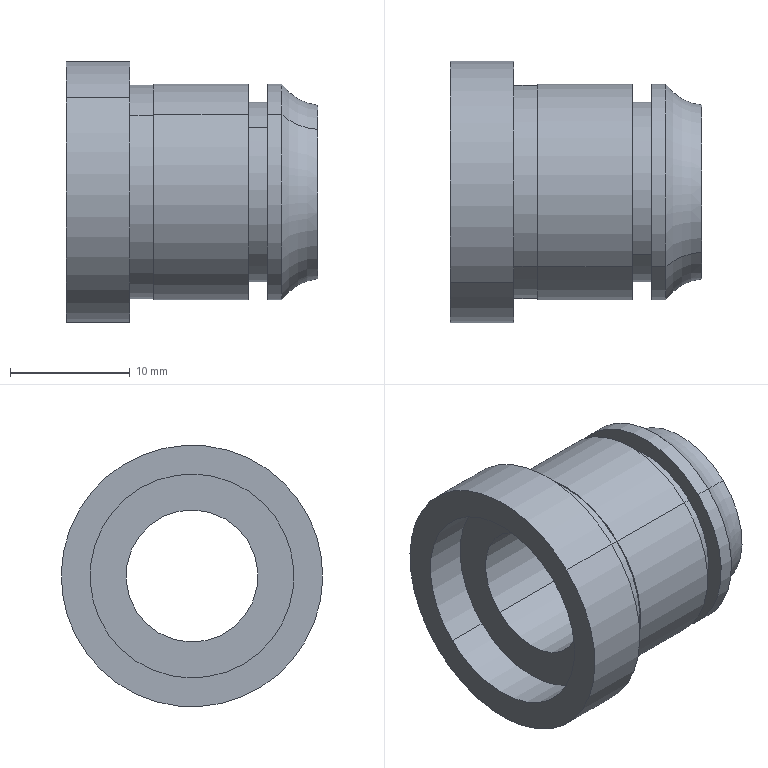Part | SolidWorks | features BaseBody 1 | 1 solid | 23 faces | box 21 x 21.8 x 21.8 mm | volume 3195 mm3 | cylinder 14 | plane 7 | torus 2 | commonest cylinder face diameters 18 x4 11 x2 15 x2 17 x2 17.8 x2 21.8 x2
STEP:
#1=CARTESIAN_POINT('',(-67.763,-3.139,-191.334));
#2=VERTEX_POINT('',#1);
#3=CARTESIAN_POINT('',(-67.763,6.932,-201.766));
#4=VERTEX_POINT('',#3);
#5=CARTESIAN_POINT('',(-67.763,1.896,-196.55));
#6=DIRECTION('',(1.,0.,0.));
#7=DIRECTION('',(0.,0.6945,-0.7195));
#8=AXIS2_PLACEMENT_3D('',#5,#6,#7);
#9=CIRCLE('',#8,7.25);
#10=EDGE_CURVE('',#2,#4,#9,.T.);
#11=ORIENTED_EDGE('',*,*,#10,.F.);
#12=CARTESIAN_POINT('',(-70.763,-4.355,-190.075));
#13=VERTEX_POINT('',#12);
#14=CARTESIAN_POINT('',(-67.447,-5.909,-188.465));
#15=DIRECTION('',(0.,0.7195,0.6945));
#16=DIRECTION('',(0.,-0.6945,0.7195));
#17=AXIS2_PLACEMENT_3D('',#14,#15,#16);
#18=CIRCLE('',#17,4.);
#19=EDGE_CURVE('',#2,#13,#18,.T.);
#20=ORIENTED_EDGE('',*,*,#19,.T.);
#21=CARTESIAN_POINT('',(-70.763,8.147,-203.025));
#22=VERTEX_POINT('',#21);
#23=CARTESIAN_POINT('',(-70.763,1.896,-196.55));
#24=DIRECTION('',(1.,0.,0.));
#25=DIRECTION('',(0.,0.6945,-0.7195));
#26=AXIS2_PLACEMENT_3D('',#23,#24,#25);
#27=CIRCLE('',#26,9.);
#28=EDGE_CURVE('',#13,#22,#27,.T.);
#29=ORIENTED_EDGE('',*,*,#28,.T.);
#30=CARTESIAN_POINT('',(-67.447,9.701,-204.635));
#31=DIRECTION('',(0.,-0.7195,-0.6945));
#32=DIRECTION('',(0.,0.6945,-0.7195));
#33=AXIS2_PLACEMENT_3D('',#30,#31,#32);
#34=CIRCLE('',#33,4.);
#35=EDGE_CURVE('',#4,#22,#34,.T.);
#36=ORIENTED_EDGE('',*,*,#35,.F.);
#37=EDGE_LOOP('',(#11,#20,#29,#36));
#38=FACE_OUTER_BOUND('',#37,.T.);
#39=CARTESIAN_POINT('',(-67.447,1.896,-196.55));
#40=DIRECTION('',(1.,0.,0.));
#41=DIRECTION('',(0.,0.6945,-0.7195));
#42=AXIS2_PLACEMENT_3D('',#39,#40,#41);
#43=TOROIDAL_SURFACE('',#42,11.238,4.);
#44=ADVANCED_FACE('',(#38),#43,.F.);
#45=CARTESIAN_POINT('',(-85.263,-1.924,-192.593));
#46=VERTEX_POINT('',#45);
#47=CARTESIAN_POINT('',(-85.263,5.716,-200.507));
#48=VERTEX_POINT('',#47);
#49=CARTESIAN_POINT('',(-85.263,1.896,-196.55));
#50=DIRECTION('',(1.,0.,0.));
#51=DIRECTION('',(0.,0.6945,-0.7195));
#52=AXIS2_PLACEMENT_3D('',#49,#50,#51);
#53=CIRCLE('',#52,5.5);
#54=EDGE_CURVE('',#46,#48,#53,.T.);
#55=ORIENTED_EDGE('',*,*,#54,.F.);
#56=CARTESIAN_POINT('',(-67.763,-1.924,-192.593));
#57=VERTEX_POINT('',#56);
#58=CARTESIAN_POINT('',(-87.763,-1.924,-192.593));
#59=DIRECTION('',(1.,0.,0.));
#60=VECTOR('',#59,1000.);
#61=LINE('',#58,#60);
#62=EDGE_CURVE('',#46,#57,#61,.T.);
#63=ORIENTED_EDGE('',*,*,#62,.T.);
#64=CARTESIAN_POINT('',(-67.763,5.716,-200.507));
#65=VERTEX_POINT('',#64);
#66=CARTESIAN_POINT('',(-67.763,1.896,-196.55));
#67=DIRECTION('',(1.,0.,0.));
#68=DIRECTION('',(0.,0.6945,-0.7195));
#69=AXIS2_PLACEMENT_3D('',#66,#67,#68);
#70=CIRCLE('',#69,5.5);
#71=EDGE_CURVE('',#57,#65,#70,.T.);
#72=ORIENTED_EDGE('',*,*,#71,.T.);
#73=CARTESIAN_POINT('',(-87.763,5.716,-200.507));
#74=DIRECTION('',(1.,0.,0.));
#75=VECTOR('',#74,1000.);
#76=LINE('',#73,#75);
#77=EDGE_CURVE('',#48,#65,#76,.T.);
#78=ORIENTED_EDGE('',*,*,#77,.F.);
#79=EDGE_LOOP('',(#55,#63,#72,#78));
#80=FACE_OUTER_BOUND('',#79,.T.);
#81=CARTESIAN_POINT('',(-87.763,1.896,-196.55));
#82=DIRECTION('',(1.,0.,0.));
#83=DIRECTION('',(0.,0.6945,-0.7195));
#84=AXIS2_PLACEMENT_3D('',#81,#82,#83);
#85=CYLINDRICAL_SURFACE('',#84,5.5);
#86=ADVANCED_FACE('',(#80),#85,.F.);
#87=CARTESIAN_POINT('',(-88.763,-4.007,-190.435));
#88=VERTEX_POINT('',#87);
#89=CARTESIAN_POINT('',(-88.763,7.8,-202.665));
#90=VERTEX_POINT('',#89);
#91=CARTESIAN_POINT('',(-88.763,1.896,-196.55));
#92=DIRECTION('',(1.,0.,0.));
#93=DIRECTION('',(0.,0.6945,-0.7195));
#94=AXIS2_PLACEMENT_3D('',#91,#92,#93);
#95=CIRCLE('',#94,8.5);
#96=EDGE_CURVE('',#88,#90,#95,.T.);
#97=ORIENTED_EDGE('',*,*,#96,.F.);
#98=CARTESIAN_POINT('',(-85.263,-4.007,-190.435));
#99=VERTEX_POINT('',#98);
#100=CARTESIAN_POINT('',(-87.763,-4.007,-190.435));
#101=DIRECTION('',(1.,0.,0.));
#102=VECTOR('',#101,1000.);
#103=LINE('',#100,#102);
#104=EDGE_CURVE('',#88,#99,#103,.T.);
#105=ORIENTED_EDGE('',*,*,#104,.T.);
#106=CARTESIAN_POINT('',(-85.263,7.8,-202.665));
#107=VERTEX_POINT('',#106);
#108=CARTESIAN_POINT('',(-85.263,1.896,-196.55));
#109=DIRECTION('',(1.,0.,0.));
#110=DIRECTION('',(0.,0.6945,-0.7195));
#111=AXIS2_PLACEMENT_3D('',#108,#109,#110);
#112=CIRCLE('',#111,8.5);
#113=EDGE_CURVE('',#99,#107,#112,.T.);
#114=ORIENTED_EDGE('',*,*,#113,.T.);
#115=CARTESIAN_POINT('',(-87.763,7.8,-202.665));
#116=DIRECTION('',(1.,0.,0.));
#117=VECTOR('',#116,1000.);
#118=LINE('',#115,#117);
#119=EDGE_CURVE('',#90,#107,#118,.T.);
#120=ORIENTED_EDGE('',*,*,#119,.F.);
#121=EDGE_LOOP('',(#97,#105,#114,#120));
#122=FACE_OUTER_BOUND('',#121,.T.);
#123=CARTESIAN_POINT('',(-87.763,1.896,-196.55));
#124=DIRECTION('',(1.,0.,0.));
#125=DIRECTION('',(0.,0.6945,-0.7195));
#126=AXIS2_PLACEMENT_3D('',#123,#124,#125);
#127=CYLINDRICAL_SURFACE('',#126,8.5);
#128=ADVANCED_FACE('',(#122),#127,.F.);
#129=CARTESIAN_POINT('',(-88.763,9.467,-204.392));
#130=VERTEX_POINT('',#129);
#131=CARTESIAN_POINT('',(-88.763,-5.674,-188.708));
#132=VERTEX_POINT('',#131);
#133=CARTESIAN_POINT('',(-88.763,1.896,-196.55));
#134=DIRECTION('',(1.,0.,0.));
#135=DIRECTION('',(0.,0.6945,-0.7195));
#136=AXIS2_PLACEMENT_3D('',#133,#134,#135);
#137=CIRCLE('',#136,10.9);
#138=EDGE_CURVE('',#130,#132,#137,.T.);
#139=ORIENTED_EDGE('',*,*,#138,.T.);
#140=CARTESIAN_POINT('',(-83.463,-5.674,-188.708));
#141=VERTEX_POINT('',#140);
#142=CARTESIAN_POINT('',(-87.763,-5.674,-188.708));
#143=DIRECTION('',(1.,0.,0.));
#144=VECTOR('',#143,1000.);
#145=LINE('',#142,#144);
#146=EDGE_CURVE('',#132,#141,#145,.T.);
#147=ORIENTED_EDGE('',*,*,#146,.T.);
#148=CARTESIAN_POINT('',(-83.463,9.467,-204.392));
#149=VERTEX_POINT('',#148);
#150=CARTESIAN_POINT('',(-83.463,1.896,-196.55));
#151=DIRECTION('',(1.,0.,0.));
#152=DIRECTION('',(0.,0.6945,-0.7195));
#153=AXIS2_PLACEMENT_3D('',#150,#151,#152);
#154=CIRCLE('',#153,10.9);
#155=EDGE_CURVE('',#149,#141,#154,.T.);
#156=ORIENTED_EDGE('',*,*,#155,.F.);
#157=CARTESIAN_POINT('',(-87.763,9.467,-204.392));
#158=DIRECTION('',(1.,0.,0.));
#159=VECTOR('',#158,1000.);
#160=LINE('',#157,#159);
#161=EDGE_CURVE('',#130,#149,#160,.T.);
#162=ORIENTED_EDGE('',*,*,#161,.F.);
#163=EDGE_LOOP('',(#139,#147,#156,#162));
#164=FACE_OUTER_BOUND('',#163,.T.);
#165=CARTESIAN_POINT('',(-87.763,1.896,-196.55));
#166=DIRECTION('',(1.,0.,0.));
#167=DIRECTION('',(0.,0.6945,-0.7195));
#168=AXIS2_PLACEMENT_3D('',#165,#166,#167);
#169=CYLINDRICAL_SURFACE('',#168,10.9);
#170=ADVANCED_FACE('',(#164),#169,.T.);
#171=CARTESIAN_POINT('',(-83.463,8.078,-202.953));
#172=VERTEX_POINT('',#171);
#173=CARTESIAN_POINT('',(-83.463,-4.285,-190.147));
#174=VERTEX_POINT('',#173);
#175=CARTESIAN_POINT('',(-83.463,1.896,-196.55));
#176=DIRECTION('',(1.,0.,0.));
#177=DIRECTION('',(0.,0.6945,-0.7195));
#178=AXIS2_PLACEMENT_3D('',#175,#176,#177);
#179=CIRCLE('',#178,8.9);
#180=EDGE_CURVE('',#172,#174,#179,.T.);
#181=ORIENTED_EDGE('',*,*,#180,.T.);
#182=CARTESIAN_POINT('',(-81.463,-4.285,-190.147));
#183=VERTEX_POINT('',#182);
#184=CARTESIAN_POINT('',(-87.763,-4.285,-190.147));
#185=DIRECTION('',(1.,0.,0.));
#186=VECTOR('',#185,1000.);
#187=LINE('',#184,#186);
#188=EDGE_CURVE('',#174,#183,#187,.T.);
#189=ORIENTED_EDGE('',*,*,#188,.T.);
#190=CARTESIAN_POINT('',(-81.463,8.078,-202.953));
#191=VERTEX_POINT('',#190);
#192=CARTESIAN_POINT('',(-81.463,1.896,-196.55));
#193=DIRECTION('',(1.,0.,0.));
#194=DIRECTION('',(0.,0.6945,-0.7195));
#195=AXIS2_PLACEMENT_3D('',#192,#193,#194);
#196=CIRCLE('',#195,8.9);
#197=EDGE_CURVE('',#191,#183,#196,.T.);
#198=ORIENTED_EDGE('',*,*,#197,.F.);
#199=CARTESIAN_POINT('',(-87.763,8.078,-202.953));
#200=DIRECTION('',(1.,0.,0.));
#201=VECTOR('',#200,1000.);
#202=LINE('',#199,#201);
#203=EDGE_CURVE('',#172,#191,#202,.T.);
#204=ORIENTED_EDGE('',*,*,#203,.F.);
#205=EDGE_LOOP('',(#181,#189,#198,#204));
#206=FACE_OUTER_BOUND('',#205,.T.);
#207=CARTESIAN_POINT('',(-87.763,1.896,-196.55));
#208=DIRECTION('',(1.,0.,0.));
#209=DIRECTION('',(0.,0.6945,-0.7195));
#210=AXIS2_PLACEMENT_3D('',#207,#208,#209);
#211=CYLINDRICAL_SURFACE('',#210,8.9);
#212=ADVANCED_FACE('',(#206),#211,.T.);
#213=CARTESIAN_POINT('',(-81.463,8.147,-203.025));
#214=VERTEX_POINT('',#213);
#215=CARTESIAN_POINT('',(-81.463,-4.355,-190.075));
#216=VERTEX_POINT('',#215);
#217=CARTESIAN_POINT('',(-81.463,1.896,-196.55));
#218=DIRECTION('',(1.,0.,0.));
#219=DIRECTION('',(0.,0.6945,-0.7195));
#220=AXIS2_PLACEMENT_3D('',#217,#218,#219);
#221=CIRCLE('',#220,9.);
#222=EDGE_CURVE('',#214,#216,#221,.T.);
#223=ORIENTED_EDGE('',*,*,#222,.T.);
#224=CARTESIAN_POINT('',(-73.563,-4.355,-190.075));
#225=VERTEX_POINT('',#224);
#226=CARTESIAN_POINT('',(-87.763,-4.355,-190.075));
#227=DIRECTION('',(1.,0.,0.));
#228=VECTOR('',#227,1000.);
#229=LINE('',#226,#228);
#230=EDGE_CURVE('',#216,#225,#229,.T.);
#231=ORIENTED_EDGE('',*,*,#230,.T.);
#232=CARTESIAN_POINT('',(-73.563,8.147,-203.025));
#233=VERTEX_POINT('',#232);
#234=CARTESIAN_POINT('',(-73.563,1.896,-196.55));
#235=DIRECTION('',(1.,0.,0.));
#236=DIRECTION('',(0.,0.6945,-0.7195));
#237=AXIS2_PLACEMENT_3D('',#234,#235,#236);
#238=CIRCLE('',#237,9.);
#239=EDGE_CURVE('',#233,#225,#238,.T.);
#240=ORIENTED_EDGE('',*,*,#239,.F.);
#241=CARTESIAN_POINT('',(-87.763,8.147,-203.025));
#242=DIRECTION('',(1.,0.,0.));
#243=VECTOR('',#242,1000.);
#244=LINE('',#241,#243);
#245=EDGE_CURVE('',#214,#233,#244,.T.);
#246=ORIENTED_EDGE('',*,*,#245,.F.);
#247=EDGE_LOOP('',(#223,#231,#240,#246));
#248=FACE_OUTER_BOUND('',#247,.T.);
#249=CARTESIAN_POINT('',(-87.763,1.896,-196.55));
#250=DIRECTION('',(1.,0.,0.));
#251=DIRECTION('',(0.,0.6945,-0.7195));
#252=AXIS2_PLACEMENT_3D('',#249,#250,#251);
#253=CYLINDRICAL_SURFACE('',#252,9.);
#254=ADVANCED_FACE('',(#248),#253,.T.);
#255=CARTESIAN_POINT('',(-73.563,7.105,-201.946));
#256=VERTEX_POINT('',#255);
#257=CARTESIAN_POINT('',(-73.563,-3.313,-191.154));
#258=VERTEX_POINT('',#257);
#259=CARTESIAN_POINT('',(-73.563,1.896,-196.55));
#260=DIRECTION('',(1.,0.,0.));
#261=DIRECTION('',(0.,0.6945,-0.7195));
#262=AXIS2_PLACEMENT_3D('',#259,#260,#261);
#263=CIRCLE('',#262,7.5);
#264=EDGE_CURVE('',#256,#258,#263,.T.);
#265=ORIENTED_EDGE('',*,*,#264,.T.);
#266=CARTESIAN_POINT('',(-71.963,-3.313,-191.154));
#267=VERTEX_POINT('',#266);
#268=CARTESIAN_POINT('',(-87.763,-3.313,-191.154));
#269=DIRECTION('',(1.,0.,0.));
#270=VECTOR('',#269,1000.);
#271=LINE('',#268,#270);
#272=EDGE_CURVE('',#258,#267,#271,.T.);
#273=ORIENTED_EDGE('',*,*,#272,.T.);
#274=CARTESIAN_POINT('',(-71.963,7.105,-201.946));
#275=VERTEX_POINT('',#274);
#276=CARTESIAN_POINT('',(-71.963,1.896,-196.55));
#277=DIRECTION('',(1.,0.,0.));
#278=DIRECTION('',(0.,0.6945,-0.7195));
#279=AXIS2_PLACEMENT_3D('',#276,#277,#278);
#280=CIRCLE('',#279,7.5);
#281=EDGE_CURVE('',#275,#267,#280,.T.);
#282=ORIENTED_EDGE('',*,*,#281,.F.);
#283=CARTESIAN_POINT('',(-87.763,7.105,-201.946));
#284=DIRECTION('',(1.,0.,0.));
#285=VECTOR('',#284,1000.);
#286=LINE('',#283,#285);
#287=EDGE_CURVE('',#256,#275,#286,.T.);
#288=ORIENTED_EDGE('',*,*,#287,.F.);
#289=EDGE_LOOP('',(#265,#273,#282,#288));
#290=FACE_OUTER_BOUND('',#289,.T.);
#291=CARTESIAN_POINT('',(-87.763,1.896,-196.55));
#292=DIRECTION('',(1.,0.,0.));
#293=DIRECTION('',(0.,0.6945,-0.7195));
#294=AXIS2_PLACEMENT_3D('',#291,#292,#293);
#295=CYLINDRICAL_SURFACE('',#294,7.5);
#296=ADVANCED_FACE('',(#290),#295,.T.);
#297=CARTESIAN_POINT('',(-71.963,8.147,-203.025));
#298=VERTEX_POINT('',#297);
#299=CARTESIAN_POINT('',(-71.963,-4.355,-190.075));
#300=VERTEX_POINT('',#299);
#301=CARTESIAN_POINT('',(-71.963,1.896,-196.55));
#302=DIRECTION('',(1.,0.,0.));
#303=DIRECTION('',(0.,0.6945,-0.7195));
#304=AXIS2_PLACEMENT_3D('',#301,#302,#303);
#305=CIRCLE('',#304,9.);
#306=EDGE_CURVE('',#298,#300,#305,.T.);
#307=ORIENTED_EDGE('',*,*,#306,.T.);
#308=CARTESIAN_POINT('',(-87.763,-4.355,-190.075));
#309=DIRECTION('',(1.,0.,0.));
#310=VECTOR('',#309,1000.);
#311=LINE('',#308,#310);
#312=EDGE_CURVE('',#300,#13,#311,.T.);
#313=ORIENTED_EDGE('',*,*,#312,.T.);
#314=CARTESIAN_POINT('',(-70.763,1.896,-196.55));
#315=DIRECTION('',(1.,0.,0.));
#316=DIRECTION('',(0.,0.6945,-0.7195));
#317=AXIS2_PLACEMENT_3D('',#314,#315,#316);
#318=CIRCLE('',#317,9.);
#319=EDGE_CURVE('',#22,#13,#318,.T.);
#320=ORIENTED_EDGE('',*,*,#319,.F.);
#321=CARTESIAN_POINT('',(-87.763,8.147,-203.025));
#322=DIRECTION('',(1.,0.,0.));
#323=VECTOR('',#322,1000.);
#324=LINE('',#321,#323);
#325=EDGE_CURVE('',#298,#22,#324,.T.);
#326=ORIENTED_EDGE('',*,*,#325,.F.);
#327=EDGE_LOOP('',(#307,#313,#320,#326));
#328=FACE_OUTER_BOUND('',#327,.T.);
#329=CARTESIAN_POINT('',(-87.763,1.896,-196.55));
#330=DIRECTION('',(1.,0.,0.));
#331=DIRECTION('',(0.,0.6945,-0.7195));
#332=AXIS2_PLACEMENT_3D('',#329,#330,#331);
#333=CYLINDRICAL_SURFACE('',#332,9.);
#334=ADVANCED_FACE('',(#328),#333,.T.);
#335=ORIENTED_EDGE('',*,*,#312,.F.);
#336=CARTESIAN_POINT('',(-71.963,1.896,-196.55));
#337=DIRECTION('',(1.,0.,0.));
#338=DIRECTION('',(0.,0.6945,-0.7195));
#339=AXIS2_PLACEMENT_3D('',#336,#337,#338);
#340=CIRCLE('',#339,9.);
#341=EDGE_CURVE('',#300,#298,#340,.T.);
#342=ORIENTED_EDGE('',*,*,#341,.T.);
#343=ORIENTED_EDGE('',*,*,#325,.T.);
#344=ORIENTED_EDGE('',*,*,#28,.F.);
#345=EDGE_LOOP('',(#335,#342,#343,#344));
#346=FACE_OUTER_BOUND('',#345,.T.);
#347=CARTESIAN_POINT('',(-87.763,1.896,-196.55));
#348=DIRECTION('',(1.,0.,0.));
#349=DIRECTION('',(0.,0.6945,-0.7195));
#350=AXIS2_PLACEMENT_3D('',#347,#348,#349);
#351=CYLINDRICAL_SURFACE('',#350,9.);
#352=ADVANCED_FACE('',(#346),#351,.T.);
#353=ORIENTED_EDGE('',*,*,#281,.T.);
#354=CARTESIAN_POINT('',(-71.963,1.896,-196.55));
#355=DIRECTION('',(1.,0.,0.));
#356=DIRECTION('',(0.,0.6945,-0.7195));
#357=AXIS2_PLACEMENT_3D('',#354,#355,#356);
#358=CIRCLE('',#357,7.5);
#359=EDGE_CURVE('',#267,#275,#358,.T.);
#360=ORIENTED_EDGE('',*,*,#359,.T.);
#361=EDGE_LOOP('',(#353,#360));
#362=FACE_BOUND('',#361,.T.);
#363=ORIENTED_EDGE('',*,*,#306,.F.);
#364=ORIENTED_EDGE('',*,*,#341,.F.);
#365=EDGE_LOOP('',(#363,#364));
#366=FACE_OUTER_BOUND('',#365,.T.);
#367=CARTESIAN_POINT('',(-71.963,7.292,-191.341));
#368=DIRECTION('',(1.,0.,0.));
#369=DIRECTION('',(0.,0.,-1.));
#370=AXIS2_PLACEMENT_3D('',#367,#368,#369);
#371=PLANE('',#370);
#372=ADVANCED_FACE('',(#362,#366),#371,.F.);
#373=ORIENTED_EDGE('',*,*,#272,.F.);
#374=CARTESIAN_POINT('',(-73.563,1.896,-196.55));
#375=DIRECTION('',(1.,0.,0.));
#376=DIRECTION('',(0.,0.6945,-0.7195));
#377=AXIS2_PLACEMENT_3D('',#374,#375,#376);
#378=CIRCLE('',#377,7.5);
#379=EDGE_CURVE('',#258,#256,#378,.T.);
#380=ORIENTED_EDGE('',*,*,#379,.T.);
#381=ORIENTED_EDGE('',*,*,#287,.T.);
#382=ORIENTED_EDGE('',*,*,#359,.F.);
#383=EDGE_LOOP('',(#373,#380,#381,#382));
#384=FACE_OUTER_BOUND('',#383,.T.);
#385=CARTESIAN_POINT('',(-87.763,1.896,-196.55));
#386=DIRECTION('',(1.,0.,0.));
#387=DIRECTION('',(0.,0.6945,-0.7195));
#388=AXIS2_PLACEMENT_3D('',#385,#386,#387);
#389=CYLINDRICAL_SURFACE('',#388,7.5);
#390=ADVANCED_FACE('',(#384),#389,.T.);
#391=ORIENTED_EDGE('',*,*,#239,.T.);
#392=CARTESIAN_POINT('',(-73.563,1.896,-196.55));
#393=DIRECTION('',(1.,0.,0.));
#394=DIRECTION('',(0.,0.6945,-0.7195));
#395=AXIS2_PLACEMENT_3D('',#392,#393,#394);
#396=CIRCLE('',#395,9.);
#397=EDGE_CURVE('',#225,#233,#396,.T.);
#398=ORIENTED_EDGE('',*,*,#397,.T.);
#399=EDGE_LOOP('',(#391,#398));
#400=FACE_OUTER_BOUND('',#399,.T.);
#401=ORIENTED_EDGE('',*,*,#264,.F.);
#402=ORIENTED_EDGE('',*,*,#379,.F.);
#403=EDGE_LOOP('',(#401,#402));
#404=FACE_BOUND('',#403,.T.);
#405=CARTESIAN_POINT('',(-73.563,8.371,-190.299));
#406=DIRECTION('',(-1.,0.,0.));
#407=DIRECTION('',(0.,1.,0.));
#408=AXIS2_PLACEMENT_3D('',#405,#406,#407);
#409=PLANE('',#408);
#410=ADVANCED_FACE('',(#400,#404),#409,.F.);
#411=ORIENTED_EDGE('',*,*,#230,.F.);
#412=CARTESIAN_POINT('',(-81.463,1.896,-196.55));
#413=DIRECTION('',(1.,0.,0.));
#414=DIRECTION('',(0.,0.6945,-0.7195));
#415=AXIS2_PLACEMENT_3D('',#412,#413,#414);
#416=CIRCLE('',#415,9.);
#417=EDGE_CURVE('',#216,#214,#416,.T.);
#418=ORIENTED_EDGE('',*,*,#417,.T.);
#419=ORIENTED_EDGE('',*,*,#245,.T.);
#420=ORIENTED_EDGE('',*,*,#397,.F.);
#421=EDGE_LOOP('',(#411,#418,#419,#420));
#422=FACE_OUTER_BOUND('',#421,.T.);
#423=CARTESIAN_POINT('',(-87.763,1.896,-196.55));
#424=DIRECTION('',(1.,0.,0.));
#425=DIRECTION('',(0.,0.6945,-0.7195));
#426=AXIS2_PLACEMENT_3D('',#423,#424,#425);
#427=CYLINDRICAL_SURFACE('',#426,9.);
#428=ADVANCED_FACE('',(#422),#427,.T.);
#429=ORIENTED_EDGE('',*,*,#197,.T.);
#430=CARTESIAN_POINT('',(-81.463,1.896,-196.55));
#431=DIRECTION('',(1.,0.,0.));
#432=DIRECTION('',(0.,0.6945,-0.7195));
#433=AXIS2_PLACEMENT_3D('',#430,#431,#432);
#434=CIRCLE('',#433,8.9);
#435=EDGE_CURVE('',#183,#191,#434,.T.);
#436=ORIENTED_EDGE('',*,*,#435,.T.);
#437=EDGE_LOOP('',(#429,#436));
#438=FACE_BOUND('',#437,.T.);
#439=ORIENTED_EDGE('',*,*,#222,.F.);
#440=ORIENTED_EDGE('',*,*,#417,.F.);
#441=EDGE_LOOP('',(#439,#440));
#442=FACE_OUTER_BOUND('',#441,.T.);
#443=CARTESIAN_POINT('',(-81.463,8.299,-190.369));
#444=DIRECTION('',(1.,0.,0.));
#445=DIRECTION('',(0.,0.,-1.));
#446=AXIS2_PLACEMENT_3D('',#443,#444,#445);
#447=PLANE('',#446);
#448=ADVANCED_FACE('',(#438,#442),#447,.F.);
#449=ORIENTED_EDGE('',*,*,#188,.F.);
#450=CARTESIAN_POINT('',(-83.463,1.896,-196.55));
#451=DIRECTION('',(1.,0.,0.));
#452=DIRECTION('',(0.,0.6945,-0.7195));
#453=AXIS2_PLACEMENT_3D('',#450,#451,#452);
#454=CIRCLE('',#453,8.9);
#455=EDGE_CURVE('',#174,#172,#454,.T.);
#456=ORIENTED_EDGE('',*,*,#455,.T.);
#457=ORIENTED_EDGE('',*,*,#203,.T.);
#458=ORIENTED_EDGE('',*,*,#435,.F.);
#459=EDGE_LOOP('',(#449,#456,#457,#458));
#460=FACE_OUTER_BOUND('',#459,.T.);
#461=CARTESIAN_POINT('',(-87.763,1.896,-196.55));
#462=DIRECTION('',(1.,0.,0.));
#463=DIRECTION('',(0.,0.6945,-0.7195));
#464=AXIS2_PLACEMENT_3D('',#461,#462,#463);
#465=CYLINDRICAL_SURFACE('',#464,8.9);
#466=ADVANCED_FACE('',(#460),#465,.T.);
#467=ORIENTED_EDGE('',*,*,#155,.T.);
#468=CARTESIAN_POINT('',(-83.463,1.896,-196.55));
#469=DIRECTION('',(1.,0.,0.));
#470=DIRECTION('',(0.,0.6945,-0.7195));
#471=AXIS2_PLACEMENT_3D('',#468,#469,#470);
#472=CIRCLE('',#471,10.9);
#473=EDGE_CURVE('',#141,#149,#472,.T.);
#474=ORIENTED_EDGE('',*,*,#473,.T.);
#475=EDGE_LOOP('',(#467,#474));
#476=FACE_OUTER_BOUND('',#475,.T.);
#477=ORIENTED_EDGE('',*,*,#180,.F.);
#478=ORIENTED_EDGE('',*,*,#455,.F.);
#479=EDGE_LOOP('',(#477,#478));
#480=FACE_BOUND('',#479,.T.);
#481=CARTESIAN_POINT('',(-83.463,9.738,-188.98));
#482=DIRECTION('',(-1.,0.,0.));
#483=DIRECTION('',(0.,1.,0.));
#484=AXIS2_PLACEMENT_3D('',#481,#482,#483);
#485=PLANE('',#484);
#486=ADVANCED_FACE('',(#476,#480),#485,.F.);
#487=ORIENTED_EDGE('',*,*,#146,.F.);
#488=CARTESIAN_POINT('',(-88.763,1.896,-196.55));
#489=DIRECTION('',(1.,0.,0.));
#490=DIRECTION('',(0.,0.6945,-0.7195));
#491=AXIS2_PLACEMENT_3D('',#488,#489,#490);
#492=CIRCLE('',#491,10.9);
#493=EDGE_CURVE('',#132,#130,#492,.T.);
#494=ORIENTED_EDGE('',*,*,#493,.T.);
#495=ORIENTED_EDGE('',*,*,#161,.T.);
#496=ORIENTED_EDGE('',*,*,#473,.F.);
#497=EDGE_LOOP('',(#487,#494,#495,#496));
#498=FACE_OUTER_BOUND('',#497,.T.);
#499=CARTESIAN_POINT('',(-87.763,1.896,-196.55));
#500=DIRECTION('',(1.,0.,0.));
#501=DIRECTION('',(0.,0.6945,-0.7195));
#502=AXIS2_PLACEMENT_3D('',#499,#500,#501);
#503=CYLINDRICAL_SURFACE('',#502,10.9);
#504=ADVANCED_FACE('',(#498),#503,.T.);
#505=CARTESIAN_POINT('',(-88.763,1.896,-196.55));
#506=DIRECTION('',(1.,0.,0.));
#507=DIRECTION('',(0.,0.6945,-0.7195));
#508=AXIS2_PLACEMENT_3D('',#505,#506,#507);
#509=CIRCLE('',#508,8.5);
#510=EDGE_CURVE('',#90,#88,#509,.T.);
#511=ORIENTED_EDGE('',*,*,#510,.T.);
#512=ORIENTED_EDGE('',*,*,#96,.T.);
#513=EDGE_LOOP('',(#511,#512));
#514=FACE_BOUND('',#513,.T.);
#515=ORIENTED_EDGE('',*,*,#138,.F.);
#516=ORIENTED_EDGE('',*,*,#493,.F.);
#517=EDGE_LOOP('',(#515,#516));
#518=FACE_OUTER_BOUND('',#517,.T.);
#519=CARTESIAN_POINT('',(-88.763,8.012,-190.646));
#520=DIRECTION('',(1.,0.,0.));
#521=DIRECTION('',(0.,0.,-1.));
#522=AXIS2_PLACEMENT_3D('',#519,#520,#521);
#523=PLANE('',#522);
#524=ADVANCED_FACE('',(#514,#518),#523,.F.);
#525=ORIENTED_EDGE('',*,*,#104,.F.);
#526=ORIENTED_EDGE('',*,*,#510,.F.);
#527=ORIENTED_EDGE('',*,*,#119,.T.);
#528=CARTESIAN_POINT('',(-85.263,1.896,-196.55));
#529=DIRECTION('',(1.,0.,0.));
#530=DIRECTION('',(0.,0.6945,-0.7195));
#531=AXIS2_PLACEMENT_3D('',#528,#529,#530);
#532=CIRCLE('',#531,8.5);
#533=EDGE_CURVE('',#107,#99,#532,.T.);
#534=ORIENTED_EDGE('',*,*,#533,.T.);
#535=EDGE_LOOP('',(#525,#526,#527,#534));
#536=FACE_OUTER_BOUND('',#535,.T.);
#537=CARTESIAN_POINT('',(-87.763,1.896,-196.55));
#538=DIRECTION('',(1.,0.,0.));
#539=DIRECTION('',(0.,0.6945,-0.7195));
#540=AXIS2_PLACEMENT_3D('',#537,#538,#539);
#541=CYLINDRICAL_SURFACE('',#540,8.5);
#542=ADVANCED_FACE('',(#536),#541,.F.);
#543=CARTESIAN_POINT('',(-85.263,1.896,-196.55));
#544=DIRECTION('',(1.,0.,0.));
#545=DIRECTION('',(0.,0.6945,-0.7195));
#546=AXIS2_PLACEMENT_3D('',#543,#544,#545);
#547=CIRCLE('',#546,5.5);
#548=EDGE_CURVE('',#48,#46,#547,.T.);
#549=ORIENTED_EDGE('',*,*,#548,.T.);
#550=ORIENTED_EDGE('',*,*,#54,.T.);
#551=EDGE_LOOP('',(#549,#550));
#552=FACE_BOUND('',#551,.T.);
#553=ORIENTED_EDGE('',*,*,#533,.F.);
#554=ORIENTED_EDGE('',*,*,#113,.F.);
#555=EDGE_LOOP('',(#553,#554));
#556=FACE_OUTER_BOUND('',#555,.T.);
#557=CARTESIAN_POINT('',(-85.263,5.853,-192.73));
#558=DIRECTION('',(1.,0.,0.));
#559=DIRECTION('',(0.,0.,-1.));
#560=AXIS2_PLACEMENT_3D('',#557,#558,#559);
#561=PLANE('',#560);
#562=ADVANCED_FACE('',(#552,#556),#561,.F.);
#563=ORIENTED_EDGE('',*,*,#62,.F.);
#564=ORIENTED_EDGE('',*,*,#548,.F.);
#565=ORIENTED_EDGE('',*,*,#77,.T.);
#566=CARTESIAN_POINT('',(-67.763,1.896,-196.55));
#567=DIRECTION('',(1.,0.,0.));
#568=DIRECTION('',(0.,0.6945,-0.7195));
#569=AXIS2_PLACEMENT_3D('',#566,#567,#568);
#570=CIRCLE('',#569,5.5);
#571=EDGE_CURVE('',#65,#57,#570,.T.);
#572=ORIENTED_EDGE('',*,*,#571,.T.);
#573=EDGE_LOOP('',(#563,#564,#565,#572));
#574=FACE_OUTER_BOUND('',#573,.T.);
#575=CARTESIAN_POINT('',(-87.763,1.896,-196.55));
#576=DIRECTION('',(1.,0.,0.));
#577=DIRECTION('',(0.,0.6945,-0.7195));
#578=AXIS2_PLACEMENT_3D('',#575,#576,#577);
#579=CYLINDRICAL_SURFACE('',#578,5.5);
#580=ADVANCED_FACE('',(#574),#579,.F.);
#581=CARTESIAN_POINT('',(-67.763,1.896,-196.55));
#582=DIRECTION('',(1.,0.,0.));
#583=DIRECTION('',(0.,0.6945,-0.7195));
#584=AXIS2_PLACEMENT_3D('',#581,#582,#583);
#585=CIRCLE('',#584,7.25);
#586=EDGE_CURVE('',#4,#2,#585,.T.);
#587=ORIENTED_EDGE('',*,*,#586,.T.);
#588=ORIENTED_EDGE('',*,*,#10,.T.);
#589=EDGE_LOOP('',(#587,#588));
#590=FACE_OUTER_BOUND('',#589,.T.);
#591=ORIENTED_EDGE('',*,*,#571,.F.);
#592=ORIENTED_EDGE('',*,*,#71,.F.);
#593=EDGE_LOOP('',(#591,#592));
#594=FACE_BOUND('',#593,.T.);
#595=CARTESIAN_POINT('',(-67.763,7.112,-191.515));
#596=DIRECTION('',(-1.,0.,0.));
#597=DIRECTION('',(0.,1.,0.));
#598=AXIS2_PLACEMENT_3D('',#595,#596,#597);
#599=PLANE('',#598);
#600=ADVANCED_FACE('',(#590,#594),#599,.F.);
#601=ORIENTED_EDGE('',*,*,#19,.F.);
#602=ORIENTED_EDGE('',*,*,#586,.F.);
#603=ORIENTED_EDGE('',*,*,#35,.T.);
#604=ORIENTED_EDGE('',*,*,#319,.T.);
#605=EDGE_LOOP('',(#601,#602,#603,#604));
#606=FACE_OUTER_BOUND('',#605,.T.);
#607=CARTESIAN_POINT('',(-67.447,1.896,-196.55));
#608=DIRECTION('',(1.,0.,0.));
#609=DIRECTION('',(0.,0.6945,-0.7195));
#610=AXIS2_PLACEMENT_3D('',#607,#608,#609);
#611=TOROIDAL_SURFACE('',#610,11.238,4.);
#612=ADVANCED_FACE('',(#606),#611,.F.);
#613=CLOSED_SHELL('',(#44,#86,#128,#170,#212,#254,#296,#334,#352,#372,#390,#410,#428,#448,#466,#486,#504,#524,#542,#562,#580,#600,#612));
#614=MANIFOLD_SOLID_BREP('',#613);
#615=CARTESIAN_POINT('',(0.,0.,0.));
#616=DIRECTION('',(0.,0.,1.));
#617=DIRECTION('',(1.,0.,0.));
#618=AXIS2_PLACEMENT_3D('',#615,#616,#617);
#619=(LENGTH_UNIT()NAMED_UNIT(*)SI_UNIT(.MILLI.,.METRE.));
#620=UNCERTAINTY_MEASURE_WITH_UNIT(LENGTH_MEASURE(0.00001),#619,'','');
#621=(NAMED_UNIT(*)PLANE_ANGLE_UNIT()SI_UNIT($,.RADIAN.));
#622=(NAMED_UNIT(*)SI_UNIT($,.STERADIAN.)SOLID_ANGLE_UNIT());
#623=(GEOMETRIC_REPRESENTATION_CONTEXT(3)GLOBAL_UNCERTAINTY_ASSIGNED_CONTEXT((#620))GLOBAL_UNIT_ASSIGNED_CONTEXT((#619,#621,#622))REPRESENTATION_CONTEXT('',''));
#624=ADVANCED_BREP_SHAPE_REPRESENTATION('',(#614,#618),#623);